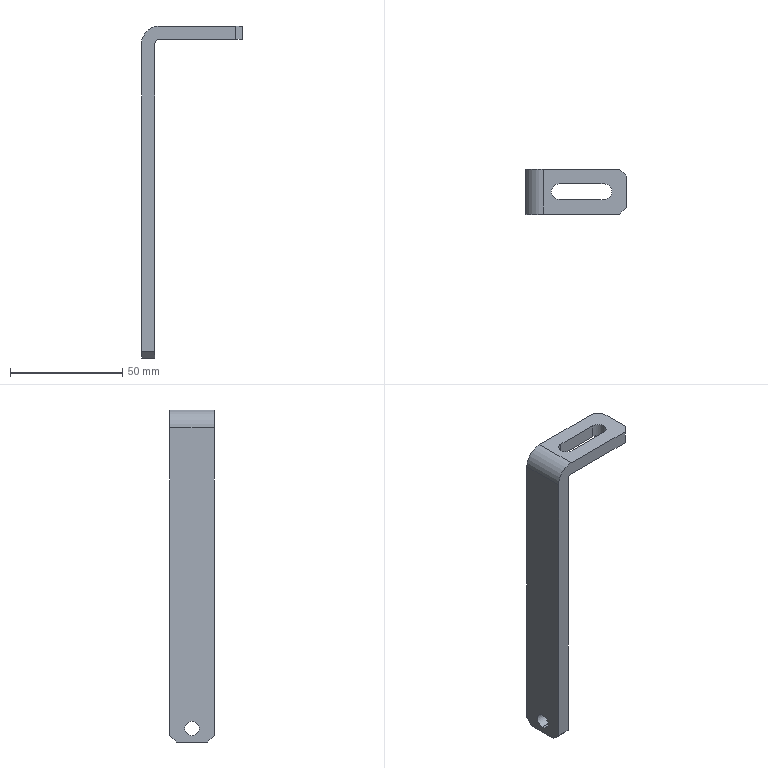Part | STEP file | PN_0024_default | 1 solid | 21 faces | box 45 x 20 x 148 mm | volume 20804 mm3 | plane 14 | cylinder 7 | commonest cylinder face diameters 7 x3 6.5 x2 4 x1 16 x1